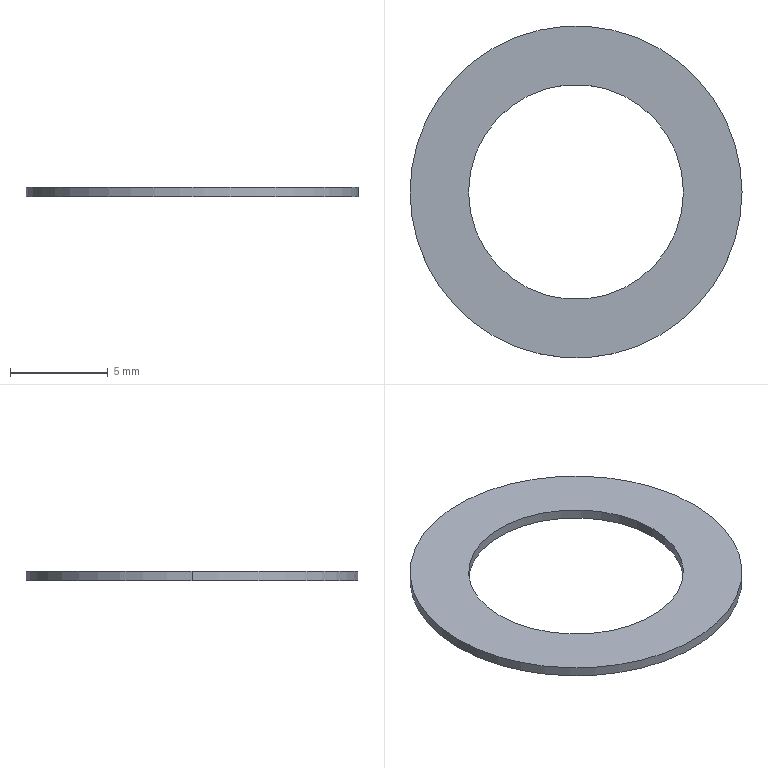Part | SolidWorks | features Extrusion 1 | 1 solid | 6 faces | box 17 x 17 x 0.5 mm | volume 65.973 mm3 | cylinder 4 | plane 2 | commonest cylinder face diameters 11 x2 17 x2
STEP:
#1=CARTESIAN_POINT('',(-5.5,0.,0.5));
#2=VERTEX_POINT('',#1);
#3=CARTESIAN_POINT('',(5.5,0.,0.5));
#4=VERTEX_POINT('',#3);
#5=CARTESIAN_POINT('',(0.,0.,0.5));
#6=DIRECTION('',(0.,0.,1.));
#7=DIRECTION('',(1.,0.,0.));
#8=AXIS2_PLACEMENT_3D('',#5,#6,#7);
#9=CIRCLE('',#8,5.5);
#10=EDGE_CURVE('',#2,#4,#9,.T.);
#11=ORIENTED_EDGE('',*,*,#10,.T.);
#12=CARTESIAN_POINT('',(5.5,0.,0.));
#13=VERTEX_POINT('',#12);
#14=CARTESIAN_POINT('',(5.5,0.,0.5));
#15=DIRECTION('',(0.,0.,-1.));
#16=VECTOR('',#15,1000.);
#17=LINE('',#14,#16);
#18=EDGE_CURVE('',#4,#13,#17,.T.);
#19=ORIENTED_EDGE('',*,*,#18,.T.);
#20=CARTESIAN_POINT('',(-5.5,0.,0.));
#21=VERTEX_POINT('',#20);
#22=CARTESIAN_POINT('',(0.,0.,0.));
#23=DIRECTION('',(0.,0.,1.));
#24=DIRECTION('',(1.,0.,0.));
#25=AXIS2_PLACEMENT_3D('',#22,#23,#24);
#26=CIRCLE('',#25,5.5);
#27=EDGE_CURVE('',#21,#13,#26,.T.);
#28=ORIENTED_EDGE('',*,*,#27,.F.);
#29=CARTESIAN_POINT('',(-5.5,0.,0.5));
#30=DIRECTION('',(0.,0.,-1.));
#31=VECTOR('',#30,1000.);
#32=LINE('',#29,#31);
#33=EDGE_CURVE('',#2,#21,#32,.T.);
#34=ORIENTED_EDGE('',*,*,#33,.F.);
#35=EDGE_LOOP('',(#11,#19,#28,#34));
#36=FACE_OUTER_BOUND('',#35,.T.);
#37=CARTESIAN_POINT('',(0.,0.,0.5));
#38=DIRECTION('',(0.,0.,-1.));
#39=DIRECTION('',(-1.,0.,0.));
#40=AXIS2_PLACEMENT_3D('',#37,#38,#39);
#41=CYLINDRICAL_SURFACE('',#40,5.5);
#42=ADVANCED_FACE('',(#36),#41,.F.);
#43=CARTESIAN_POINT('',(8.5,0.,0.5));
#44=VERTEX_POINT('',#43);
#45=CARTESIAN_POINT('',(-8.5,0.,0.5));
#46=VERTEX_POINT('',#45);
#47=CARTESIAN_POINT('',(0.,0.,0.5));
#48=DIRECTION('',(0.,0.,1.));
#49=DIRECTION('',(1.,0.,0.));
#50=AXIS2_PLACEMENT_3D('',#47,#48,#49);
#51=CIRCLE('',#50,8.5);
#52=EDGE_CURVE('',#44,#46,#51,.T.);
#53=ORIENTED_EDGE('',*,*,#52,.F.);
#54=CARTESIAN_POINT('',(8.5,0.,0.));
#55=VERTEX_POINT('',#54);
#56=CARTESIAN_POINT('',(8.5,0.,0.5));
#57=DIRECTION('',(0.,0.,-1.));
#58=VECTOR('',#57,1000.);
#59=LINE('',#56,#58);
#60=EDGE_CURVE('',#44,#55,#59,.T.);
#61=ORIENTED_EDGE('',*,*,#60,.T.);
#62=CARTESIAN_POINT('',(-8.5,0.,0.));
#63=VERTEX_POINT('',#62);
#64=CARTESIAN_POINT('',(0.,0.,0.));
#65=DIRECTION('',(0.,0.,1.));
#66=DIRECTION('',(1.,0.,0.));
#67=AXIS2_PLACEMENT_3D('',#64,#65,#66);
#68=CIRCLE('',#67,8.5);
#69=EDGE_CURVE('',#55,#63,#68,.T.);
#70=ORIENTED_EDGE('',*,*,#69,.T.);
#71=CARTESIAN_POINT('',(-8.5,0.,0.5));
#72=DIRECTION('',(0.,0.,-1.));
#73=VECTOR('',#72,1000.);
#74=LINE('',#71,#73);
#75=EDGE_CURVE('',#46,#63,#74,.T.);
#76=ORIENTED_EDGE('',*,*,#75,.F.);
#77=EDGE_LOOP('',(#53,#61,#70,#76));
#78=FACE_OUTER_BOUND('',#77,.T.);
#79=CARTESIAN_POINT('',(0.,0.,0.5));
#80=DIRECTION('',(0.,0.,-1.));
#81=DIRECTION('',(-1.,0.,0.));
#82=AXIS2_PLACEMENT_3D('',#79,#80,#81);
#83=CYLINDRICAL_SURFACE('',#82,8.5);
#84=ADVANCED_FACE('',(#78),#83,.T.);
#85=CARTESIAN_POINT('',(0.,0.,0.5));
#86=DIRECTION('',(0.,0.,1.));
#87=DIRECTION('',(1.,0.,0.));
#88=AXIS2_PLACEMENT_3D('',#85,#86,#87);
#89=CIRCLE('',#88,8.5);
#90=EDGE_CURVE('',#46,#44,#89,.T.);
#91=ORIENTED_EDGE('',*,*,#90,.T.);
#92=ORIENTED_EDGE('',*,*,#52,.T.);
#93=EDGE_LOOP('',(#91,#92));
#94=FACE_OUTER_BOUND('',#93,.T.);
#95=ORIENTED_EDGE('',*,*,#10,.F.);
#96=CARTESIAN_POINT('',(0.,0.,0.5));
#97=DIRECTION('',(0.,0.,1.));
#98=DIRECTION('',(1.,0.,0.));
#99=AXIS2_PLACEMENT_3D('',#96,#97,#98);
#100=CIRCLE('',#99,5.5);
#101=EDGE_CURVE('',#4,#2,#100,.T.);
#102=ORIENTED_EDGE('',*,*,#101,.F.);
#103=EDGE_LOOP('',(#95,#102));
#104=FACE_BOUND('',#103,.T.);
#105=CARTESIAN_POINT('',(0.,0.,0.5));
#106=DIRECTION('',(0.,0.,1.));
#107=DIRECTION('',(1.,0.,0.));
#108=AXIS2_PLACEMENT_3D('',#105,#106,#107);
#109=PLANE('',#108);
#110=ADVANCED_FACE('',(#94,#104),#109,.T.);
#111=CARTESIAN_POINT('',(0.,0.,0.));
#112=DIRECTION('',(0.,0.,1.));
#113=DIRECTION('',(1.,0.,0.));
#114=AXIS2_PLACEMENT_3D('',#111,#112,#113);
#115=CIRCLE('',#114,8.5);
#116=EDGE_CURVE('',#63,#55,#115,.T.);
#117=ORIENTED_EDGE('',*,*,#116,.F.);
#118=ORIENTED_EDGE('',*,*,#69,.F.);
#119=EDGE_LOOP('',(#117,#118));
#120=FACE_OUTER_BOUND('',#119,.T.);
#121=ORIENTED_EDGE('',*,*,#27,.T.);
#122=CARTESIAN_POINT('',(0.,0.,0.));
#123=DIRECTION('',(0.,0.,1.));
#124=DIRECTION('',(1.,0.,0.));
#125=AXIS2_PLACEMENT_3D('',#122,#123,#124);
#126=CIRCLE('',#125,5.5);
#127=EDGE_CURVE('',#13,#21,#126,.T.);
#128=ORIENTED_EDGE('',*,*,#127,.T.);
#129=EDGE_LOOP('',(#121,#128));
#130=FACE_BOUND('',#129,.T.);
#131=CARTESIAN_POINT('',(0.,0.,0.));
#132=DIRECTION('',(0.,0.,1.));
#133=DIRECTION('',(1.,0.,0.));
#134=AXIS2_PLACEMENT_3D('',#131,#132,#133);
#135=PLANE('',#134);
#136=ADVANCED_FACE('',(#120,#130),#135,.F.);
#137=ORIENTED_EDGE('',*,*,#60,.F.);
#138=ORIENTED_EDGE('',*,*,#90,.F.);
#139=ORIENTED_EDGE('',*,*,#75,.T.);
#140=ORIENTED_EDGE('',*,*,#116,.T.);
#141=EDGE_LOOP('',(#137,#138,#139,#140));
#142=FACE_OUTER_BOUND('',#141,.T.);
#143=CARTESIAN_POINT('',(0.,0.,0.5));
#144=DIRECTION('',(0.,0.,-1.));
#145=DIRECTION('',(-1.,0.,0.));
#146=AXIS2_PLACEMENT_3D('',#143,#144,#145);
#147=CYLINDRICAL_SURFACE('',#146,8.5);
#148=ADVANCED_FACE('',(#142),#147,.T.);
#149=ORIENTED_EDGE('',*,*,#18,.F.);
#150=ORIENTED_EDGE('',*,*,#101,.T.);
#151=ORIENTED_EDGE('',*,*,#33,.T.);
#152=ORIENTED_EDGE('',*,*,#127,.F.);
#153=EDGE_LOOP('',(#149,#150,#151,#152));
#154=FACE_OUTER_BOUND('',#153,.T.);
#155=CARTESIAN_POINT('',(0.,0.,0.5));
#156=DIRECTION('',(0.,0.,-1.));
#157=DIRECTION('',(-1.,0.,0.));
#158=AXIS2_PLACEMENT_3D('',#155,#156,#157);
#159=CYLINDRICAL_SURFACE('',#158,5.5);
#160=ADVANCED_FACE('',(#154),#159,.F.);
#161=CLOSED_SHELL('',(#42,#84,#110,#136,#148,#160));
#162=MANIFOLD_SOLID_BREP('',#161);
#163=CARTESIAN_POINT('',(0.,0.,0.));
#164=DIRECTION('',(0.,0.,1.));
#165=DIRECTION('',(1.,0.,0.));
#166=AXIS2_PLACEMENT_3D('',#163,#164,#165);
#167=(LENGTH_UNIT()NAMED_UNIT(*)SI_UNIT(.MILLI.,.METRE.));
#168=UNCERTAINTY_MEASURE_WITH_UNIT(LENGTH_MEASURE(0.00001),#167,'','');
#169=(NAMED_UNIT(*)PLANE_ANGLE_UNIT()SI_UNIT($,.RADIAN.));
#170=(NAMED_UNIT(*)SI_UNIT($,.STERADIAN.)SOLID_ANGLE_UNIT());
#171=(GEOMETRIC_REPRESENTATION_CONTEXT(3)GLOBAL_UNCERTAINTY_ASSIGNED_CONTEXT((#168))GLOBAL_UNIT_ASSIGNED_CONTEXT((#167,#169,#170))REPRESENTATION_CONTEXT('',''));
#172=ADVANCED_BREP_SHAPE_REPRESENTATION('',(#162,#166),#171);